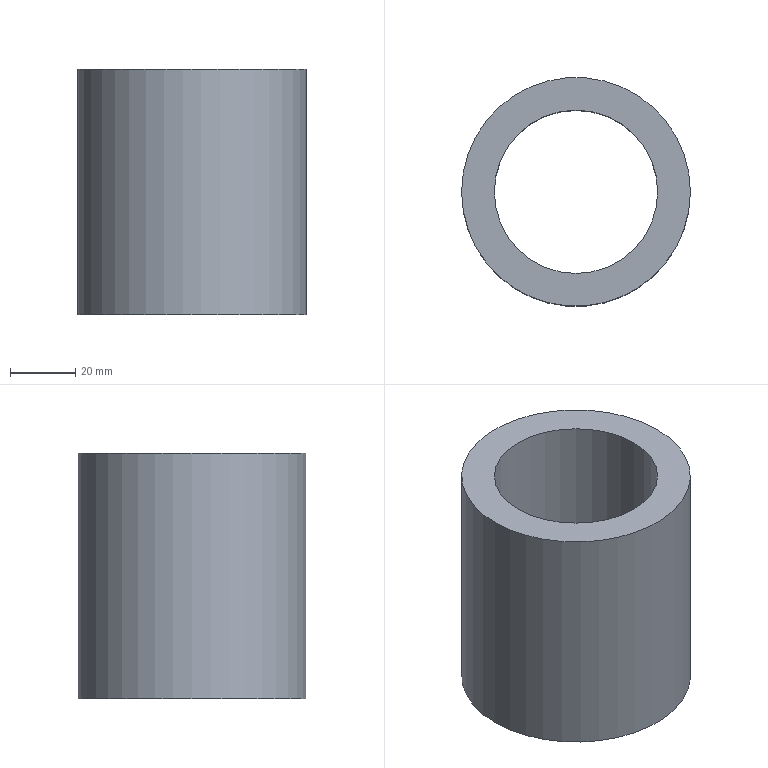Part | NX | features solid 2 | 1 solid | 4 faces | box 70 x 70 x 75 mm | volume 141372 mm3 | cylinder 2 | plane 2 | commonest cylinder face diameters 50 x1 70 x1
STEP:
#1=CARTESIAN_POINT('',(-395.,-220.,-175.));
#2=VERTEX_POINT('',#1);
#3=CARTESIAN_POINT('',(-420.,-220.,-175.));
#4=DIRECTION('',(0.,0.,-1.));
#5=DIRECTION('',(1.,0.,0.));
#6=AXIS2_PLACEMENT_3D('',#3,#4,#5);
#7=CIRCLE('',#6,25.);
#8=EDGE_CURVE('',#2,#2,#7,.T.);
#9=ORIENTED_EDGE('',*,*,#8,.F.);
#10=EDGE_LOOP('',(#9));
#11=FACE_BOUND('',#10,.T.);
#12=CARTESIAN_POINT('',(-395.,-220.,-250.));
#13=VERTEX_POINT('',#12);
#14=CARTESIAN_POINT('',(-420.,-220.,-250.));
#15=DIRECTION('',(0.,0.,-1.));
#16=DIRECTION('',(1.,0.,0.));
#17=AXIS2_PLACEMENT_3D('',#14,#15,#16);
#18=CIRCLE('',#17,25.);
#19=EDGE_CURVE('',#13,#13,#18,.T.);
#20=ORIENTED_EDGE('',*,*,#19,.T.);
#21=EDGE_LOOP('',(#20));
#22=FACE_BOUND('',#21,.T.);
#23=CARTESIAN_POINT('',(-420.,-220.,-175.));
#24=DIRECTION('',(0.,0.,-1.));
#25=DIRECTION('',(-1.,0.,0.));
#26=AXIS2_PLACEMENT_3D('',#23,#24,#25);
#27=CYLINDRICAL_SURFACE('',#26,25.);
#28=ADVANCED_FACE('',(#11,#22),#27,.F.);
#29=CARTESIAN_POINT('',(-385.,-220.,-175.));
#30=VERTEX_POINT('',#29);
#31=CARTESIAN_POINT('',(-420.,-220.,-175.));
#32=DIRECTION('',(0.,0.,-1.));
#33=DIRECTION('',(1.,0.,0.));
#34=AXIS2_PLACEMENT_3D('',#31,#32,#33);
#35=CIRCLE('',#34,35.);
#36=EDGE_CURVE('',#30,#30,#35,.T.);
#37=ORIENTED_EDGE('',*,*,#36,.T.);
#38=EDGE_LOOP('',(#37));
#39=FACE_BOUND('',#38,.T.);
#40=CARTESIAN_POINT('',(-385.,-220.,-250.));
#41=VERTEX_POINT('',#40);
#42=CARTESIAN_POINT('',(-420.,-220.,-250.));
#43=DIRECTION('',(0.,0.,-1.));
#44=DIRECTION('',(1.,0.,0.));
#45=AXIS2_PLACEMENT_3D('',#42,#43,#44);
#46=CIRCLE('',#45,35.);
#47=EDGE_CURVE('',#41,#41,#46,.T.);
#48=ORIENTED_EDGE('',*,*,#47,.F.);
#49=EDGE_LOOP('',(#48));
#50=FACE_BOUND('',#49,.T.);
#51=CARTESIAN_POINT('',(-420.,-220.,-175.));
#52=DIRECTION('',(0.,0.,-1.));
#53=DIRECTION('',(-1.,0.,0.));
#54=AXIS2_PLACEMENT_3D('',#51,#52,#53);
#55=CYLINDRICAL_SURFACE('',#54,35.);
#56=ADVANCED_FACE('',(#39,#50),#55,.T.);
#57=ORIENTED_EDGE('',*,*,#8,.T.);
#58=EDGE_LOOP('',(#57));
#59=FACE_BOUND('',#58,.T.);
#60=ORIENTED_EDGE('',*,*,#36,.F.);
#61=EDGE_LOOP('',(#60));
#62=FACE_BOUND('',#61,.T.);
#63=CARTESIAN_POINT('',(-420.,-220.,-175.));
#64=DIRECTION('',(0.,0.,1.));
#65=DIRECTION('',(1.,0.,0.));
#66=AXIS2_PLACEMENT_3D('',#63,#64,#65);
#67=PLANE('',#66);
#68=ADVANCED_FACE('',(#59,#62),#67,.T.);
#69=ORIENTED_EDGE('',*,*,#19,.F.);
#70=EDGE_LOOP('',(#69));
#71=FACE_BOUND('',#70,.T.);
#72=ORIENTED_EDGE('',*,*,#47,.T.);
#73=EDGE_LOOP('',(#72));
#74=FACE_BOUND('',#73,.T.);
#75=CARTESIAN_POINT('',(-420.,-220.,-250.));
#76=DIRECTION('',(0.,0.,1.));
#77=DIRECTION('',(1.,0.,0.));
#78=AXIS2_PLACEMENT_3D('',#75,#76,#77);
#79=PLANE('',#78);
#80=ADVANCED_FACE('',(#71,#74),#79,.F.);
#81=CLOSED_SHELL('',(#28,#56,#68,#80));
#82=MANIFOLD_SOLID_BREP('',#81);
#83=(LENGTH_UNIT()NAMED_UNIT(*)SI_UNIT(.MILLI.,.METRE.));
#84=UNCERTAINTY_MEASURE_WITH_UNIT(LENGTH_MEASURE(0.00001),#83,'','');
#85=(NAMED_UNIT(*)PLANE_ANGLE_UNIT()SI_UNIT($,.RADIAN.));
#86=(NAMED_UNIT(*)SI_UNIT($,.STERADIAN.)SOLID_ANGLE_UNIT());
#87=(GEOMETRIC_REPRESENTATION_CONTEXT(3)GLOBAL_UNCERTAINTY_ASSIGNED_CONTEXT((#84))GLOBAL_UNIT_ASSIGNED_CONTEXT((#83,#85,#86))REPRESENTATION_CONTEXT('',''));
#88=ADVANCED_BREP_SHAPE_REPRESENTATION('',(#82),#87);